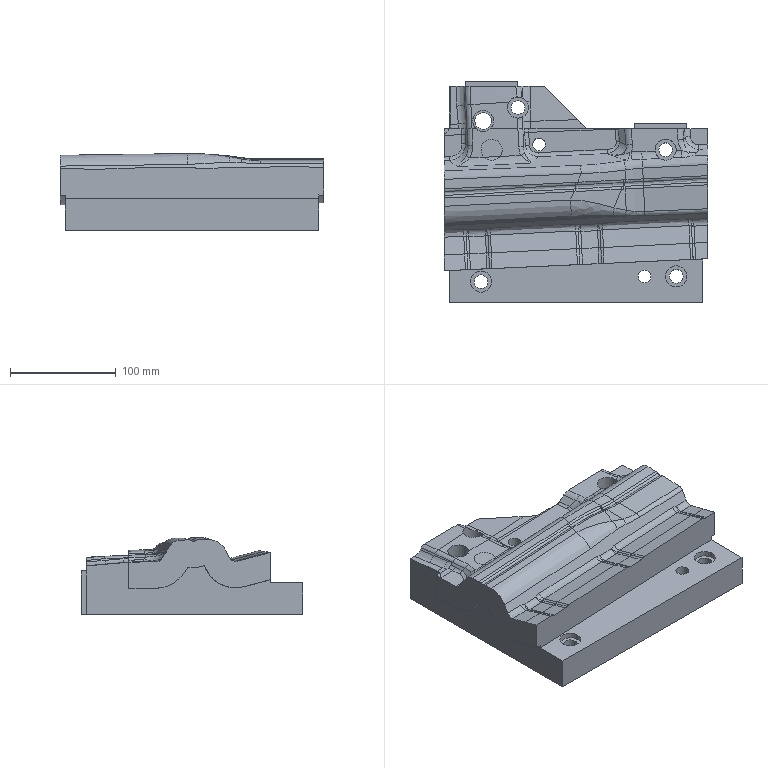Part | NX | features solid 2 | 1 solid | 216 faces | box 250 x 210 x 72.901 mm | volume 2372289 mm3 | spline 176 | plane 27 | cylinder 13 | commonest cylinder face diameters 20 x5 13 x4 12 x2 16 x1 23 x1